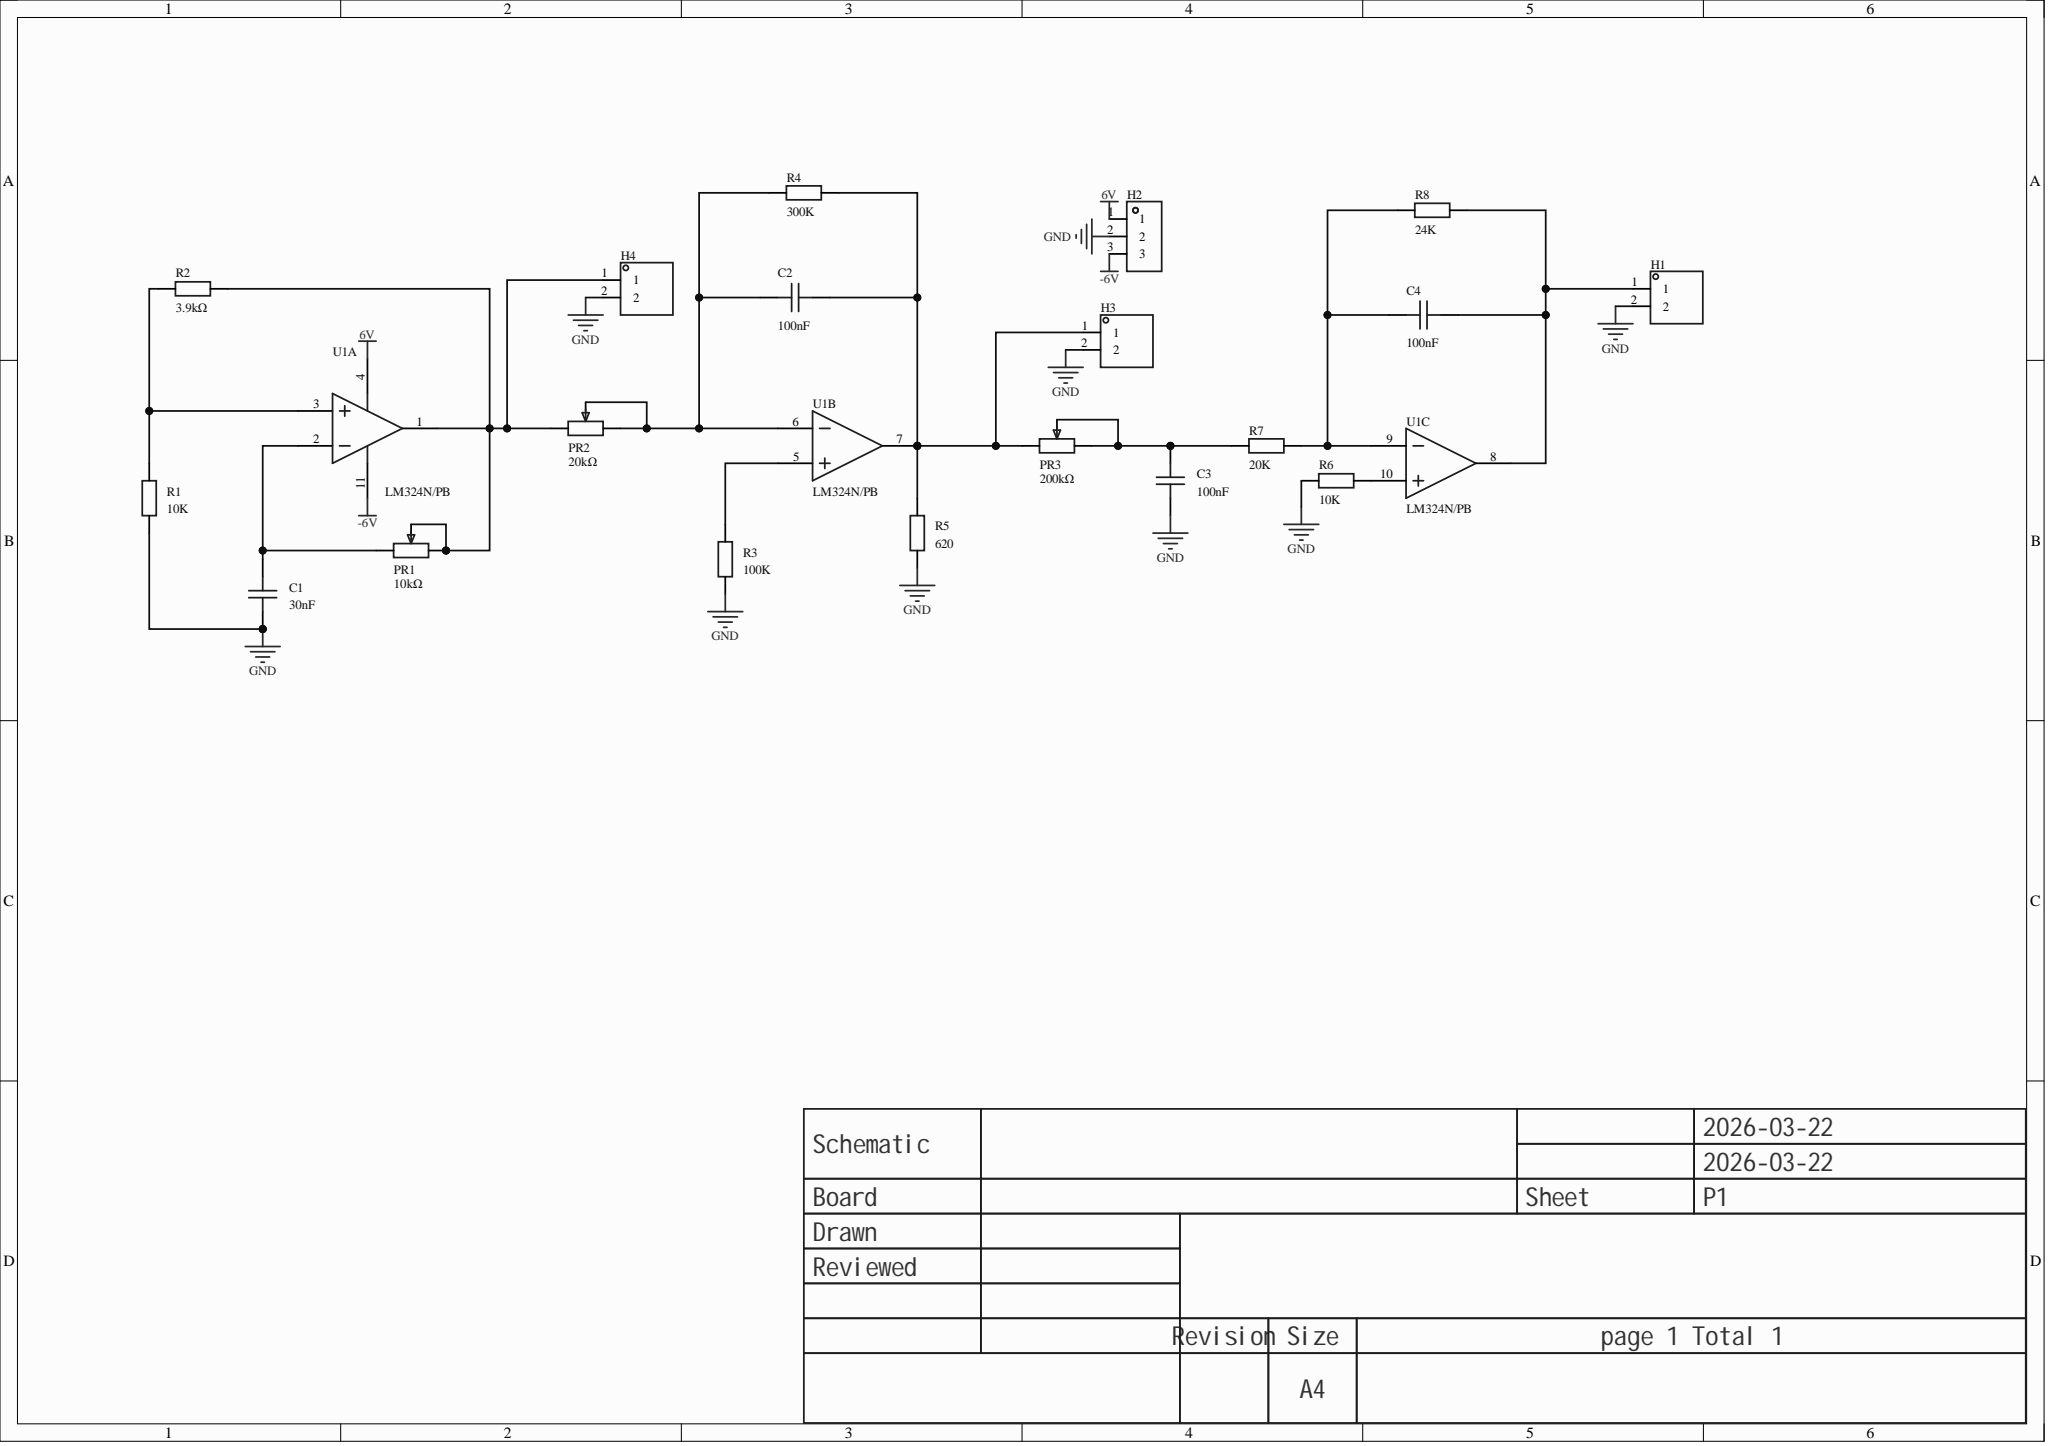Circuit board | Altium Designer | 20 parts | 13 nets
Bill of materials:
Comment,Description,Designator,Footprint,LibRef,Quantity
"30nF","","C1","C0603","CAP_0603","1"
"100nF","","C2, C3, C4","C0603","CAP_0603","3"
"","","H1, H3, H4","HDR-TH_2P-P2.54-V-M-1","HDR-M_2.54_1x2P","3"
"","","H2","HDR-TH_3P-P2.54-V-M","HDR-M_2.54_1x3P","1"
"10kΩ","","PR1","R_3296","R_3296","1"
"20kΩ","","PR2","R_3296","R_3296","1"
"200kΩ","","PR3","R_3296","R_3296","1"
"10K","","R1, R6","R0603","Res_0603","2"
"3.9kΩ","","R2","R0603","Res_0603","1"
"100K","","R3","R0603","Res_0603","1"
"300K","","R4","R0603","Res_0603","1"
"620","","R5","R0603","Res_0603","1"
"20K","","R7","R0603","Res_0603","1"
"24K","","R8","R0603","Res_0603","1"
"LM324N/PB","LM324N/PB component. Amplifiers: quad; gain-bandwidth product (GBP): 1MHz; input bias current (Ib): 45nA;","U1","PDIP-14_L19.2-W6.6-P2.54-LS7.6-BL","LM324N/PB","1"
Netlist (Protel format):
[
C1
C0603
30nF



]
[
C2
C0603
100nF



]
[
C3
C0603
100nF



]
[
C4
C0603
100nF



]
[
H1
HDR-TH_2P-P2.54-V-M-1




]
[
H2
HDR-TH_3P-P2.54-V-M




]
[
H3
HDR-TH_2P-P2.54-V-M-1




]
[
H4
HDR-TH_2P-P2.54-V-M-1




]
[
PR1
R_3296
10kΩ



]
[
PR2
R_3296
20kΩ



]
[
PR3
R_3296
200kΩ



]
[
R1
R0603
10K



]
[
R2
R0603
3.9kΩ



]
[
R3
R0603
100K



]
[
R4
R0603
300K



]
[
R5
R0603
620



]
[
R6
R0603
10K



]
[
R7
R0603
20K



]
[
R8
R0603
24K



]
[
U1
PDIP-14_L19.2-W6.6-P2.54-LS7.6-BL
LM324N/PB



]
(
NetR6_2
R6-2
U1-10
)
(
NetR3_2
R3-2
U1-5
)
(
NetR1_2
R1-2
R2-2
U1-3
)
(
NetH4_1
H4-1
PR1-1
PR1-2
PR2-3
R2-1
U1-1
)
(
NetC4_2
C4-2
H1-1
R8-2
U1-8
)
(
NetC4_1
C4-1
R7-2
R8-1
U1-9
)
(
NetC3_2
C3-2
PR3-1
PR3-2
R7-1
)
(
NetC2_2
C2-2
H3-1
PR3-3
R4-2
R5-2
U1-7
)
(
NetC2_1
C2-1
PR2-1
PR2-2
R4-1
U1-6
)
(
NetC1_2
C1-2
PR1-3
U1-2
)
(
GND
C1-1
C3-1
H1-2
H2-2
H3-2
H4-2
R1-1
R3-1
R5-1
R6-1
)
(
-6V
H2-3
U1-11
)
(
6V
H2-1
U1-4
)